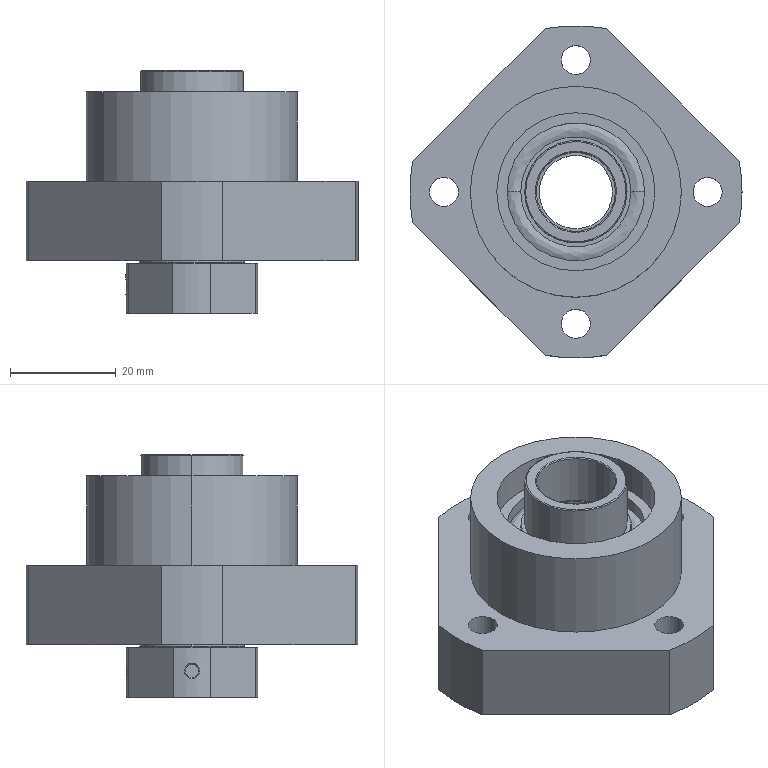Part | SolidWorks | features BaseBody 1 | 1 solid | 128 faces | box 63 x 63 x 46 mm | volume 51941 mm3 | cylinder 62 | spline 28 | plane 28 | cone 10 | commonest cylinder face diameters 5.5 x8 9.5 x8 15 x8 32 x6 25 x5 63 x5